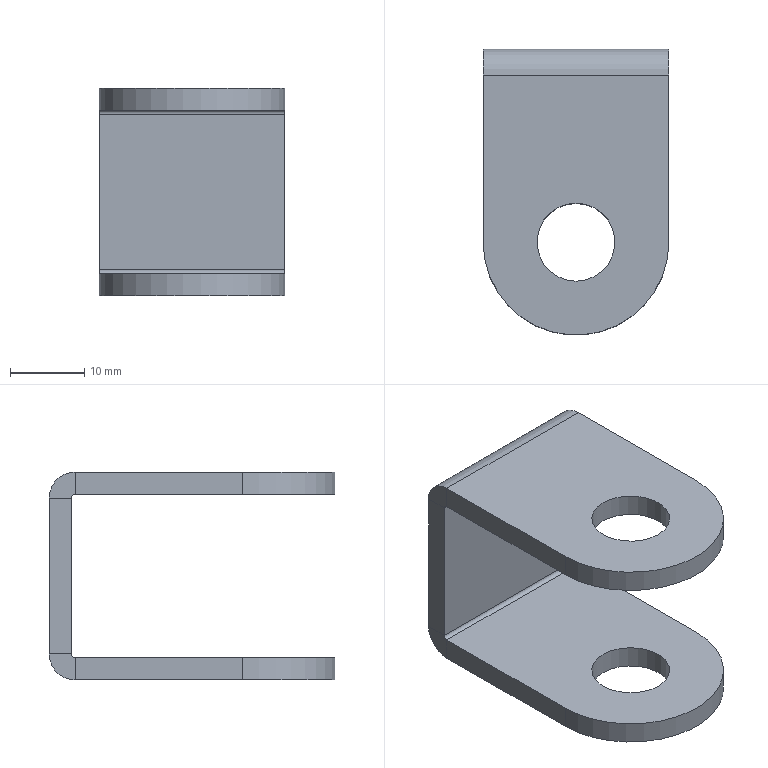Part | STEP file | Q7C0106 | 1 solid | 24 faces | box 25 x 38.5 x 28 mm | volume 6374 mm3 | plane 16 | cylinder 8 | commonest cylinder face diameters 1 x2 7 x2 10.5 x2 25 x2